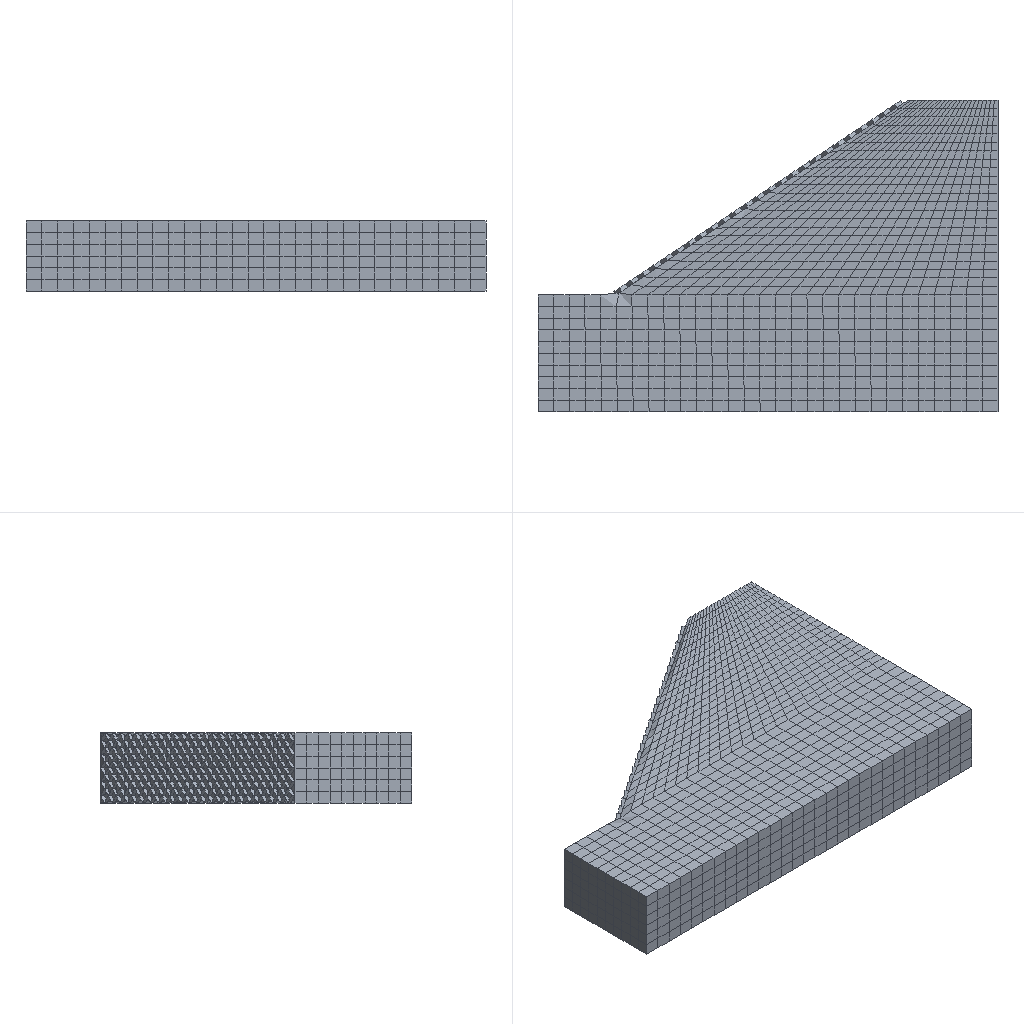Simulation study | abaqus
Set-up summary:
category,name,step,type,value,unit,region
solver,abaqus
solver,version,,,Abaqus/Standard 2020
units,not stated in the deck,,not stated
analysis,deck,,static,static
load_step,Step-load,Step-load,static,nlgeom=True
load_step,Step-reduce,Step-reduce,static,nlgeom=True
contact,interactions,,,general=0 pairs=0 ties=1
load_step,requested,,,2
mesh,nodes,,,6895
mesh,elements,,,5552
element_type,S4R,,shell,500
element_type,C3D8R,,solid,5052
load,load commands in deck,,count,2
bc,support commands in deck,,count,3
material,G,,in results
material,MATERIAL-1,,in results
check,setup vs results,,match,"per instance, exact: element labels, types and connectivity; labels of the nodes the elements use; coordinates of those nodes at SINGLE_PRECISION in 1 of 2 instance(s)"
Abaqus input file, long lists of numbers shortened:
*Heading
** Job name: Job-1 Model name: Model-1
** Generated by: Abaqus/CAE 2020
*Preprint, echo=NO, model=NO, history=NO, contact=NO
**
** PARTS
**
*Part, name=qiao
*Node
      1,   1.414,  -1.515,  0.1
      2,    1.237,   -1.338,  0.1
** (558 more lines like these left out)
*Element, type=S4R
1, 1, 2, 3, 4
2, 2, 5, 6, 3
** (498 more lines like these left out)
*Nset, nset=Set-1, generate
   1,  560,    1
*Elset, elset=Set-1, generate
   1,  500,    1
** Section: g
*Shell Section, elset=Set-1, material=g
0.01, 5
*End Part
**
*Part, name=soil
*Node
      1,   11.802,           0.,   1.8
      2,   11.802,           0.,           0.
** (6333 more lines like these left out)
*Element, type=C3D8R
   1,  168, 1562, 2546,  550,    1,   15,  330,   68
   2, 1562, 1563, 2547, 2546,   15,   16,  331,  330
** (5050 more lines like these left out)
*Nset, nset=Set-1, generate
    1,  6335,     1
*Elset, elset=Set-1, generate
    1,  5052,     1
** Section: soil
*Solid Section, elset=Set-1, material=Material-1
,
*End Part
**
**
** ASSEMBLY
**
*Assembly, name=Assembly
**
*Instance, name=soil-1, part=soil
*End Instance
**
*Instance, name=qiao-1, part=qiao
10.265, 5.63,     1.607
10.265, 5.63,     1.607, 10.692, 6.428, 1.18, 102.865
*End Instance
**
*Nset, nset=Set-2, instance=soil-1
    9,   10,   12,   13,  224,  225,  226,  227,  228,  252,  253,  254,  255,  256,  266,  267
  268,  269,  270,  271,  272,  273,  274,  275,  276,  277,  278,  279,  280,  281,  282,  283
** (12 more lines like these left out)
*Elset, elset=Set-2, instance=soil-1
 3367, 3368, 3369, 3370, 3371, 3372, 3427, 3428, 3429, 3430, 3431, 3432, 3487, 3488, 3489, 3490
 3491, 3492, 3547, 3548, 3549, 3550, 3551, 3552, 3607, 3608, 3609, 3610, 3611, 3612, 3667, 3668
** (9 more lines like these left out)
*Nset, nset=Set-3, instance=soil-1
    1,    2,    3,    4,    5,    6,    7,    8,    9,   10,   11,   12,   13,   14,   20,   21
   22,   23,   24,   25,   26,   27,   28,   29,   30,   31,   32,   33,   34,   35,   36,   37
** (112 more lines like these left out)
*Elset, elset=Set-3, instance=soil-1
    1,    6,    7,   12,   13,   18,   19,   24,   25,   30,   31,   36,   37,   42,   43,   48
   49,   54,   55,   60,   61,   66,   67,   72,   73,   78,   79,   84,   85,   90,   91,   96
** (104 more lines like these left out)
*Nset, nset=Set-4, instance=soil-1
    1,    2,    3,    4,    9,   10,   11,   12,   13,   14,   15,   16,   17,   18,   19,   20
   21,   22,   23,   24,   25,   26,   27,   28,   29,   30,   31,   32,   33,   34,   35,   36
** (18 more lines like these left out)
*Elset, elset=Set-4, instance=soil-1
    1,    2,    3,    4,    5,    6,    7,    8,    9,   10,   11,   12,   13,   14,   15,   16
   17,   18,   19,   20,   21,   22,   23,   24,   25,   26,   27,   28,   29,   30,   31,   32
** (15 more lines like these left out)
*Nset, nset=Set-5, instance=soil-1, generate
    1,  6335,     1
*Nset, nset=Set-5, instance=qiao-1, generate
   1,  560,    1
*Elset, elset=Set-5, instance=soil-1, generate
    1,  5052,     1
*Elset, elset=Set-5, instance=qiao-1, generate
   1,  500,    1
*Nset, nset=m_Set-1, instance=qiao-1
   1,   2,   5,   7,   9,  10,  13,  15,  16,  19,  21,  22,  25,  27,  29,  31
  32,  35,  37,  38,  41,  42,  45,  47,  49,  51,  52,  55,  57,  58,  61,  62
** (16 more lines like these left out)
*Elset, elset=m_Set-1, instance=qiao-1, generate
   1,  500,    1
*Elset, elset=_m_Surf-1_E1, internal, instance=qiao-1
 157, 160, 163, 164, 185, 188, 189, 192, 203, 205, 206, 207, 208, 209, 210, 211
 212, 237, 240, 241, 242, 243, 244, 245, 246, 247, 248, 249, 250, 251, 252
*Surface, type=ELEMENT, name=m_Surf-1
_m_Surf-1_E1, E1
*Elset, elset=_s_Surf-1_S1, internal, instance=soil-1, generate
 3175,  3312,     1
*Surface, type=ELEMENT, name=s_Surf-1
_s_Surf-1_S1, S1
*Surface, type=NODE, name=m_Set-1_CNS_, internal
m_Set-1, 1.
** Constraint: Constraint-1
*Tie, name=Constraint-1, adjust=yes, type=NODE TO SURFACE
s_Surf-1, m_Set-1_CNS_
*End Assembly
*Amplitude, name=Amp-1
             0.,              0.,             0.1,            -18.,             0.2,              0.,             0.3,            -24.
            0.4,              0.,             0.5,            -18.,             0.6,              0.,             0.7,            -20.
            0.8,              0.,             0.9,            -18.,              1.,              0.
**
** MATERIALS
**
*Material, name=Material-1
*Density
2000.,
*Elastic
 3.5e+08, 0.3
*Expansion
 1e-06,
*Mohr Coulomb, dependencies=1
 35.52,  0.1, ,  0.5
   31.,  0.1, , 0.75
   28.,  0.1, ,   1.
   24.,  0.1, , 1.25
   20.,  0.1, ,  1.5
   19.,  0.1, , 1.75
   18.,  0.1, ,   2.
*Mohr Coulomb Hardening, dependencies=1
18450.,   0., ,  0.5
15000.,   0., , 0.75
12500.,   0., ,   1.
 9000.,   0., , 1.25
 8000.,   0., ,  1.5
 6000.,   0., , 1.75
 4000.,   0., ,   2.
*Material, name=g
*Density
2700.,
*Elastic
29531., 0.22
*Expansion
 1e-05,
** ----------------------------------------------------------------
*initial conditions,type=field,variable=1
soil-1.Set-1,0.5
**
** STEP: Step-load
**
*Step, name=Step-load, nlgeom=YES, inc=1000, unsymm=YES
*Static
0.01, 1., 1e-05, 0.1
**
** BOUNDARY CONDITIONS
**
** Name: BC-1 Type: 位移/转角
*Boundary
Set-2, 2, 2
** Name: [REDACTED] : Displacement/rotation angle
*Boundary
Set-4, 1, 1
** Name: [REDACTED] : Displacement/rotation angle
*Boundary
Set-3, 3, 3
**
** LOADS
**
** Name: Load-1   Type: Gravity
*Dload
, GRAV, 0.1, 0., -1., 0.
**
** PREDEFINED FIELDS
**
** Name: Predefined Field-1   Type: Temperature
*Temperature, amplitude=Amp-1
Set-5, 1.
**
** OUTPUT REQUESTS
**
*Restart, write, frequency=0
**
** FIELD OUTPUT: F-Output-1
**
*Output, field
*Node Output
CF, NT, RF, U, V
*Element Output, directions=YES
E, FV, LE, MISES, MISESONLY, PE, PEEQ, PEEQMAX, PEEQT, PEMAG, PRESSONLY, S, SEQUT, SSAVG, TEMP, YIELDPOT
*Contact Output
CDISP, CSTRESS
**
** HISTORY OUTPUT: H-Output-1
**
*Output, history, variable=PRESELECT
*End Step
** ----------------------------------------------------------------
**
** STEP: Step-reduce
**
*Step, name=Step-reduce, nlgeom=YES, inc=1000, unsymm=YES
*Static
0.01, 1., 1e-05, 0.1
*field,variable=1
soil-1.Set-1,2
**
** OUTPUT REQUESTS
**
*Restart, write, frequency=0
**
** FIELD OUTPUT: F-Output-1
**
*Output, field
*Node Output
CF, NT, RF, U, V
*Element Output, directions=YES
E, FV, LE, MISES, MISESONLY, PE, PEEQ, PEEQMAX, PEEQT, PEMAG, PRESSONLY, S, SEQUT, SSAVG, TEMP, YIELDPOT
*Contact Output
CDISP, CSTRESS
**
** HISTORY OUTPUT: H-Output-1
**
*Output, history, variable=PRESELECT
*End Step
Results summary:
result,step,,completed,increments=17 time=1.0/1.0
result,step,,completed,increments=15 time=1.0/1.0
result,analysis,,,static
result,last_loadstep,,,2
result,analysis steps,,count,2
result,primary field,,,"U, UR"
result,reaction total,,FX,-1.7e-05,model units
result,reaction total,,FY,23657.7,model units
result,reaction total,,FZ,0.0,model units